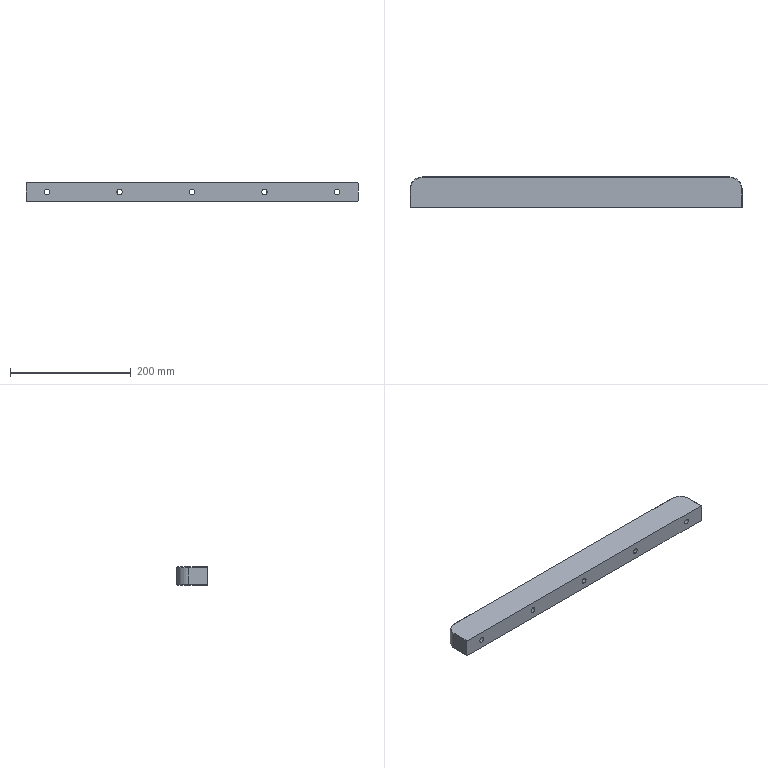Part | STEP file | TJ-DHQM-003-013 | 1 solid | 43 faces | box 550 x 50 x 30 mm | volume 789176 mm3 | cylinder 22 | plane 17 | cone 4 | commonest cylinder face diameters 9 x10 15 x10 40 x2
STEP:
#1=CARTESIAN_POINT('',(240.,25.,-7.5));
#2=VERTEX_POINT('',#1);
#3=CARTESIAN_POINT('',(240.,25.,7.5));
#4=VERTEX_POINT('',#3);
#5=CARTESIAN_POINT('',(240.,25.,0.));
#6=DIRECTION('',(0.,1.,0.));
#7=DIRECTION('',(0.,0.,1.));
#8=AXIS2_PLACEMENT_3D('',#5,#6,#7);
#9=CIRCLE('',#8,7.5);
#10=EDGE_CURVE('',#2,#4,#9,.T.);
#11=ORIENTED_EDGE('',*,*,#10,.F.);
#12=CARTESIAN_POINT('',(240.,50.,-7.5));
#13=VERTEX_POINT('',#12);
#14=CARTESIAN_POINT('',(240.,50.,-7.5));
#15=DIRECTION('',(0.,1.,0.));
#16=VECTOR('',#15,1000.);
#17=LINE('',#14,#16);
#18=EDGE_CURVE('',#2,#13,#17,.T.);
#19=ORIENTED_EDGE('',*,*,#18,.T.);
#20=CARTESIAN_POINT('',(240.,50.,7.5));
#21=VERTEX_POINT('',#20);
#22=CARTESIAN_POINT('',(240.,50.,0.));
#23=DIRECTION('',(0.,1.,0.));
#24=DIRECTION('',(0.,0.,1.));
#25=AXIS2_PLACEMENT_3D('',#22,#23,#24);
#26=CIRCLE('',#25,7.5);
#27=EDGE_CURVE('',#13,#21,#26,.T.);
#28=ORIENTED_EDGE('',*,*,#27,.T.);
#29=CARTESIAN_POINT('',(240.,50.,7.5));
#30=DIRECTION('',(0.,1.,0.));
#31=VECTOR('',#30,1000.);
#32=LINE('',#29,#31);
#33=EDGE_CURVE('',#4,#21,#32,.T.);
#34=ORIENTED_EDGE('',*,*,#33,.F.);
#35=EDGE_LOOP('',(#11,#19,#28,#34));
#36=FACE_OUTER_BOUND('',#35,.T.);
#37=CARTESIAN_POINT('',(240.,50.,0.));
#38=DIRECTION('',(0.,1.,0.));
#39=DIRECTION('',(0.,0.,1.));
#40=AXIS2_PLACEMENT_3D('',#37,#38,#39);
#41=CYLINDRICAL_SURFACE('',#40,7.5);
#42=ADVANCED_FACE('',(#36),#41,.F.);
#43=CARTESIAN_POINT('',(240.,0.,-4.5));
#44=VERTEX_POINT('',#43);
#45=CARTESIAN_POINT('',(240.,0.,4.5));
#46=VERTEX_POINT('',#45);
#47=CARTESIAN_POINT('',(240.,0.,0.));
#48=DIRECTION('',(0.,1.,0.));
#49=DIRECTION('',(0.,0.,1.));
#50=AXIS2_PLACEMENT_3D('',#47,#48,#49);
#51=CIRCLE('',#50,4.5);
#52=EDGE_CURVE('',#44,#46,#51,.T.);
#53=ORIENTED_EDGE('',*,*,#52,.F.);
#54=CARTESIAN_POINT('',(240.,25.,-4.5));
#55=VERTEX_POINT('',#54);
#56=CARTESIAN_POINT('',(240.,50.,-4.5));
#57=DIRECTION('',(0.,1.,0.));
#58=VECTOR('',#57,1000.);
#59=LINE('',#56,#58);
#60=EDGE_CURVE('',#44,#55,#59,.T.);
#61=ORIENTED_EDGE('',*,*,#60,.T.);
#62=CARTESIAN_POINT('',(240.,25.,4.5));
#63=VERTEX_POINT('',#62);
#64=CARTESIAN_POINT('',(240.,25.,0.));
#65=DIRECTION('',(0.,1.,0.));
#66=DIRECTION('',(0.,0.,1.));
#67=AXIS2_PLACEMENT_3D('',#64,#65,#66);
#68=CIRCLE('',#67,4.5);
#69=EDGE_CURVE('',#55,#63,#68,.T.);
#70=ORIENTED_EDGE('',*,*,#69,.T.);
#71=CARTESIAN_POINT('',(240.,50.,4.5));
#72=DIRECTION('',(0.,1.,0.));
#73=VECTOR('',#72,1000.);
#74=LINE('',#71,#73);
#75=EDGE_CURVE('',#46,#63,#74,.T.);
#76=ORIENTED_EDGE('',*,*,#75,.F.);
#77=EDGE_LOOP('',(#53,#61,#70,#76));
#78=FACE_OUTER_BOUND('',#77,.T.);
#79=CARTESIAN_POINT('',(240.,50.,0.));
#80=DIRECTION('',(0.,1.,0.));
#81=DIRECTION('',(0.,0.,1.));
#82=AXIS2_PLACEMENT_3D('',#79,#80,#81);
#83=CYLINDRICAL_SURFACE('',#82,4.5);
#84=ADVANCED_FACE('',(#78),#83,.F.);
#85=CARTESIAN_POINT('',(120.,25.,-7.5));
#86=VERTEX_POINT('',#85);
#87=CARTESIAN_POINT('',(120.,25.,7.5));
#88=VERTEX_POINT('',#87);
#89=CARTESIAN_POINT('',(120.,25.,0.));
#90=DIRECTION('',(0.,1.,0.));
#91=DIRECTION('',(0.,0.,1.));
#92=AXIS2_PLACEMENT_3D('',#89,#90,#91);
#93=CIRCLE('',#92,7.5);
#94=EDGE_CURVE('',#86,#88,#93,.T.);
#95=ORIENTED_EDGE('',*,*,#94,.F.);
#96=CARTESIAN_POINT('',(120.,50.,-7.5));
#97=VERTEX_POINT('',#96);
#98=CARTESIAN_POINT('',(120.,50.,-7.5));
#99=DIRECTION('',(0.,1.,0.));
#100=VECTOR('',#99,1000.);
#101=LINE('',#98,#100);
#102=EDGE_CURVE('',#86,#97,#101,.T.);
#103=ORIENTED_EDGE('',*,*,#102,.T.);
#104=CARTESIAN_POINT('',(120.,50.,7.5));
#105=VERTEX_POINT('',#104);
#106=CARTESIAN_POINT('',(120.,50.,0.));
#107=DIRECTION('',(0.,1.,0.));
#108=DIRECTION('',(0.,0.,1.));
#109=AXIS2_PLACEMENT_3D('',#106,#107,#108);
#110=CIRCLE('',#109,7.5);
#111=EDGE_CURVE('',#97,#105,#110,.T.);
#112=ORIENTED_EDGE('',*,*,#111,.T.);
#113=CARTESIAN_POINT('',(120.,50.,7.5));
#114=DIRECTION('',(0.,1.,0.));
#115=VECTOR('',#114,1000.);
#116=LINE('',#113,#115);
#117=EDGE_CURVE('',#88,#105,#116,.T.);
#118=ORIENTED_EDGE('',*,*,#117,.F.);
#119=EDGE_LOOP('',(#95,#103,#112,#118));
#120=FACE_OUTER_BOUND('',#119,.T.);
#121=CARTESIAN_POINT('',(120.,50.,0.));
#122=DIRECTION('',(0.,1.,0.));
#123=DIRECTION('',(0.,0.,1.));
#124=AXIS2_PLACEMENT_3D('',#121,#122,#123);
#125=CYLINDRICAL_SURFACE('',#124,7.5);
#126=ADVANCED_FACE('',(#120),#125,.F.);
#127=CARTESIAN_POINT('',(120.,0.,-4.5));
#128=VERTEX_POINT('',#127);
#129=CARTESIAN_POINT('',(120.,0.,4.5));
#130=VERTEX_POINT('',#129);
#131=CARTESIAN_POINT('',(120.,0.,0.));
#132=DIRECTION('',(0.,1.,0.));
#133=DIRECTION('',(0.,0.,1.));
#134=AXIS2_PLACEMENT_3D('',#131,#132,#133);
#135=CIRCLE('',#134,4.5);
#136=EDGE_CURVE('',#128,#130,#135,.T.);
#137=ORIENTED_EDGE('',*,*,#136,.F.);
#138=CARTESIAN_POINT('',(120.,25.,-4.5));
#139=VERTEX_POINT('',#138);
#140=CARTESIAN_POINT('',(120.,50.,-4.5));
#141=DIRECTION('',(0.,1.,0.));
#142=VECTOR('',#141,1000.);
#143=LINE('',#140,#142);
#144=EDGE_CURVE('',#128,#139,#143,.T.);
#145=ORIENTED_EDGE('',*,*,#144,.T.);
#146=CARTESIAN_POINT('',(120.,25.,4.5));
#147=VERTEX_POINT('',#146);
#148=CARTESIAN_POINT('',(120.,25.,0.));
#149=DIRECTION('',(0.,1.,0.));
#150=DIRECTION('',(0.,0.,1.));
#151=AXIS2_PLACEMENT_3D('',#148,#149,#150);
#152=CIRCLE('',#151,4.5);
#153=EDGE_CURVE('',#139,#147,#152,.T.);
#154=ORIENTED_EDGE('',*,*,#153,.T.);
#155=CARTESIAN_POINT('',(120.,50.,4.5));
#156=DIRECTION('',(0.,1.,0.));
#157=VECTOR('',#156,1000.);
#158=LINE('',#155,#157);
#159=EDGE_CURVE('',#130,#147,#158,.T.);
#160=ORIENTED_EDGE('',*,*,#159,.F.);
#161=EDGE_LOOP('',(#137,#145,#154,#160));
#162=FACE_OUTER_BOUND('',#161,.T.);
#163=CARTESIAN_POINT('',(120.,50.,0.));
#164=DIRECTION('',(0.,1.,0.));
#165=DIRECTION('',(0.,0.,1.));
#166=AXIS2_PLACEMENT_3D('',#163,#164,#165);
#167=CYLINDRICAL_SURFACE('',#166,4.5);
#168=ADVANCED_FACE('',(#162),#167,.F.);
#169=CARTESIAN_POINT('',(-240.,25.,-7.5));
#170=VERTEX_POINT('',#169);
#171=CARTESIAN_POINT('',(-240.,25.,7.5));
#172=VERTEX_POINT('',#171);
#173=CARTESIAN_POINT('',(-240.,25.,0.));
#174=DIRECTION('',(0.,1.,0.));
#175=DIRECTION('',(0.,0.,1.));
#176=AXIS2_PLACEMENT_3D('',#173,#174,#175);
#177=CIRCLE('',#176,7.5);
#178=EDGE_CURVE('',#170,#172,#177,.T.);
#179=ORIENTED_EDGE('',*,*,#178,.F.);
#180=CARTESIAN_POINT('',(-240.,50.,-7.5));
#181=VERTEX_POINT('',#180);
#182=CARTESIAN_POINT('',(-240.,50.,-7.5));
#183=DIRECTION('',(0.,1.,0.));
#184=VECTOR('',#183,1000.);
#185=LINE('',#182,#184);
#186=EDGE_CURVE('',#170,#181,#185,.T.);
#187=ORIENTED_EDGE('',*,*,#186,.T.);
#188=CARTESIAN_POINT('',(-240.,50.,7.5));
#189=VERTEX_POINT('',#188);
#190=CARTESIAN_POINT('',(-240.,50.,0.));
#191=DIRECTION('',(0.,1.,0.));
#192=DIRECTION('',(0.,0.,1.));
#193=AXIS2_PLACEMENT_3D('',#190,#191,#192);
#194=CIRCLE('',#193,7.5);
#195=EDGE_CURVE('',#181,#189,#194,.T.);
#196=ORIENTED_EDGE('',*,*,#195,.T.);
#197=CARTESIAN_POINT('',(-240.,50.,7.5));
#198=DIRECTION('',(0.,1.,0.));
#199=VECTOR('',#198,1000.);
#200=LINE('',#197,#199);
#201=EDGE_CURVE('',#172,#189,#200,.T.);
#202=ORIENTED_EDGE('',*,*,#201,.F.);
#203=EDGE_LOOP('',(#179,#187,#196,#202));
#204=FACE_OUTER_BOUND('',#203,.T.);
#205=CARTESIAN_POINT('',(-240.,50.,0.));
#206=DIRECTION('',(0.,1.,0.));
#207=DIRECTION('',(0.,0.,1.));
#208=AXIS2_PLACEMENT_3D('',#205,#206,#207);
#209=CYLINDRICAL_SURFACE('',#208,7.5);
#210=ADVANCED_FACE('',(#204),#209,.F.);
#211=CARTESIAN_POINT('',(-240.,0.,-4.5));
#212=VERTEX_POINT('',#211);
#213=CARTESIAN_POINT('',(-240.,0.,4.5));
#214=VERTEX_POINT('',#213);
#215=CARTESIAN_POINT('',(-240.,0.,0.));
#216=DIRECTION('',(0.,1.,0.));
#217=DIRECTION('',(0.,0.,1.));
#218=AXIS2_PLACEMENT_3D('',#215,#216,#217);
#219=CIRCLE('',#218,4.5);
#220=EDGE_CURVE('',#212,#214,#219,.T.);
#221=ORIENTED_EDGE('',*,*,#220,.F.);
#222=CARTESIAN_POINT('',(-240.,25.,-4.5));
#223=VERTEX_POINT('',#222);
#224=CARTESIAN_POINT('',(-240.,50.,-4.5));
#225=DIRECTION('',(0.,1.,0.));
#226=VECTOR('',#225,1000.);
#227=LINE('',#224,#226);
#228=EDGE_CURVE('',#212,#223,#227,.T.);
#229=ORIENTED_EDGE('',*,*,#228,.T.);
#230=CARTESIAN_POINT('',(-240.,25.,4.5));
#231=VERTEX_POINT('',#230);
#232=CARTESIAN_POINT('',(-240.,25.,0.));
#233=DIRECTION('',(0.,1.,0.));
#234=DIRECTION('',(0.,0.,1.));
#235=AXIS2_PLACEMENT_3D('',#232,#233,#234);
#236=CIRCLE('',#235,4.5);
#237=EDGE_CURVE('',#223,#231,#236,.T.);
#238=ORIENTED_EDGE('',*,*,#237,.T.);
#239=CARTESIAN_POINT('',(-240.,50.,4.5));
#240=DIRECTION('',(0.,1.,0.));
#241=VECTOR('',#240,1000.);
#242=LINE('',#239,#241);
#243=EDGE_CURVE('',#214,#231,#242,.T.);
#244=ORIENTED_EDGE('',*,*,#243,.F.);
#245=EDGE_LOOP('',(#221,#229,#238,#244));
#246=FACE_OUTER_BOUND('',#245,.T.);
#247=CARTESIAN_POINT('',(-240.,50.,0.));
#248=DIRECTION('',(0.,1.,0.));
#249=DIRECTION('',(0.,0.,1.));
#250=AXIS2_PLACEMENT_3D('',#247,#248,#249);
#251=CYLINDRICAL_SURFACE('',#250,4.5);
#252=ADVANCED_FACE('',(#246),#251,.F.);
#253=CARTESIAN_POINT('',(-120.,25.,-7.5));
#254=VERTEX_POINT('',#253);
#255=CARTESIAN_POINT('',(-120.,25.,7.5));
#256=VERTEX_POINT('',#255);
#257=CARTESIAN_POINT('',(-120.,25.,0.));
#258=DIRECTION('',(0.,1.,0.));
#259=DIRECTION('',(0.,0.,1.));
#260=AXIS2_PLACEMENT_3D('',#257,#258,#259);
#261=CIRCLE('',#260,7.5);
#262=EDGE_CURVE('',#254,#256,#261,.T.);
#263=ORIENTED_EDGE('',*,*,#262,.F.);
#264=CARTESIAN_POINT('',(-120.,50.,-7.5));
#265=VERTEX_POINT('',#264);
#266=CARTESIAN_POINT('',(-120.,50.,-7.5));
#267=DIRECTION('',(0.,1.,0.));
#268=VECTOR('',#267,1000.);
#269=LINE('',#266,#268);
#270=EDGE_CURVE('',#254,#265,#269,.T.);
#271=ORIENTED_EDGE('',*,*,#270,.T.);
#272=CARTESIAN_POINT('',(-120.,50.,7.5));
#273=VERTEX_POINT('',#272);
#274=CARTESIAN_POINT('',(-120.,50.,0.));
#275=DIRECTION('',(0.,1.,0.));
#276=DIRECTION('',(0.,0.,1.));
#277=AXIS2_PLACEMENT_3D('',#274,#275,#276);
#278=CIRCLE('',#277,7.5);
#279=EDGE_CURVE('',#265,#273,#278,.T.);
#280=ORIENTED_EDGE('',*,*,#279,.T.);
#281=CARTESIAN_POINT('',(-120.,50.,7.5));
#282=DIRECTION('',(0.,1.,0.));
#283=VECTOR('',#282,1000.);
#284=LINE('',#281,#283);
#285=EDGE_CURVE('',#256,#273,#284,.T.);
#286=ORIENTED_EDGE('',*,*,#285,.F.);
#287=EDGE_LOOP('',(#263,#271,#280,#286));
#288=FACE_OUTER_BOUND('',#287,.T.);
#289=CARTESIAN_POINT('',(-120.,50.,0.));
#290=DIRECTION('',(0.,1.,0.));
#291=DIRECTION('',(0.,0.,1.));
#292=AXIS2_PLACEMENT_3D('',#289,#290,#291);
#293=CYLINDRICAL_SURFACE('',#292,7.5);
#294=ADVANCED_FACE('',(#288),#293,.F.);
#295=CARTESIAN_POINT('',(-120.,0.,-4.5));
#296=VERTEX_POINT('',#295);
#297=CARTESIAN_POINT('',(-120.,0.,4.5));
#298=VERTEX_POINT('',#297);
#299=CARTESIAN_POINT('',(-120.,0.,0.));
#300=DIRECTION('',(0.,1.,0.));
#301=DIRECTION('',(0.,0.,1.));
#302=AXIS2_PLACEMENT_3D('',#299,#300,#301);
#303=CIRCLE('',#302,4.5);
#304=EDGE_CURVE('',#296,#298,#303,.T.);
#305=ORIENTED_EDGE('',*,*,#304,.F.);
#306=CARTESIAN_POINT('',(-120.,25.,-4.5));
#307=VERTEX_POINT('',#306);
#308=CARTESIAN_POINT('',(-120.,50.,-4.5));
#309=DIRECTION('',(0.,1.,0.));
#310=VECTOR('',#309,1000.);
#311=LINE('',#308,#310);
#312=EDGE_CURVE('',#296,#307,#311,.T.);
#313=ORIENTED_EDGE('',*,*,#312,.T.);
#314=CARTESIAN_POINT('',(-120.,25.,4.5));
#315=VERTEX_POINT('',#314);
#316=CARTESIAN_POINT('',(-120.,25.,0.));
#317=DIRECTION('',(0.,1.,0.));
#318=DIRECTION('',(0.,0.,1.));
#319=AXIS2_PLACEMENT_3D('',#316,#317,#318);
#320=CIRCLE('',#319,4.5);
#321=EDGE_CURVE('',#307,#315,#320,.T.);
#322=ORIENTED_EDGE('',*,*,#321,.T.);
#323=CARTESIAN_POINT('',(-120.,50.,4.5));
#324=DIRECTION('',(0.,1.,0.));
#325=VECTOR('',#324,1000.);
#326=LINE('',#323,#325);
#327=EDGE_CURVE('',#298,#315,#326,.T.);
#328=ORIENTED_EDGE('',*,*,#327,.F.);
#329=EDGE_LOOP('',(#305,#313,#322,#328));
#330=FACE_OUTER_BOUND('',#329,.T.);
#331=CARTESIAN_POINT('',(-120.,50.,0.));
#332=DIRECTION('',(0.,1.,0.));
#333=DIRECTION('',(0.,0.,1.));
#334=AXIS2_PLACEMENT_3D('',#331,#332,#333);
#335=CYLINDRICAL_SURFACE('',#334,4.5);
#336=ADVANCED_FACE('',(#330),#335,.F.);
#337=CARTESIAN_POINT('',(0.,25.,-7.5));
#338=VERTEX_POINT('',#337);
#339=CARTESIAN_POINT('',(0.,25.,7.5));
#340=VERTEX_POINT('',#339);
#341=CARTESIAN_POINT('',(0.,25.,0.));
#342=DIRECTION('',(0.,1.,0.));
#343=DIRECTION('',(0.,0.,1.));
#344=AXIS2_PLACEMENT_3D('',#341,#342,#343);
#345=CIRCLE('',#344,7.5);
#346=EDGE_CURVE('',#338,#340,#345,.T.);
#347=ORIENTED_EDGE('',*,*,#346,.F.);
#348=CARTESIAN_POINT('',(0.,50.,-7.5));
#349=VERTEX_POINT('',#348);
#350=CARTESIAN_POINT('',(0.,50.,-7.5));
#351=DIRECTION('',(0.,1.,0.));
#352=VECTOR('',#351,1000.);
#353=LINE('',#350,#352);
#354=EDGE_CURVE('',#338,#349,#353,.T.);
#355=ORIENTED_EDGE('',*,*,#354,.T.);
#356=CARTESIAN_POINT('',(0.,50.,7.5));
#357=VERTEX_POINT('',#356);
#358=CARTESIAN_POINT('',(0.,50.,0.));
#359=DIRECTION('',(0.,1.,0.));
#360=DIRECTION('',(0.,0.,1.));
#361=AXIS2_PLACEMENT_3D('',#358,#359,#360);
#362=CIRCLE('',#361,7.5);
#363=EDGE_CURVE('',#349,#357,#362,.T.);
#364=ORIENTED_EDGE('',*,*,#363,.T.);
#365=CARTESIAN_POINT('',(0.,50.,7.5));
#366=DIRECTION('',(0.,1.,0.));
#367=VECTOR('',#366,1000.);
#368=LINE('',#365,#367);
#369=EDGE_CURVE('',#340,#357,#368,.T.);
#370=ORIENTED_EDGE('',*,*,#369,.F.);
#371=EDGE_LOOP('',(#347,#355,#364,#370));
#372=FACE_OUTER_BOUND('',#371,.T.);
#373=CARTESIAN_POINT('',(0.,50.,0.));
#374=DIRECTION('',(0.,1.,0.));
#375=DIRECTION('',(0.,0.,1.));
#376=AXIS2_PLACEMENT_3D('',#373,#374,#375);
#377=CYLINDRICAL_SURFACE('',#376,7.5);
#378=ADVANCED_FACE('',(#372),#377,.F.);
#379=CARTESIAN_POINT('',(0.,0.,-4.5));
#380=VERTEX_POINT('',#379);
#381=CARTESIAN_POINT('',(0.,0.,4.5));
#382=VERTEX_POINT('',#381);
#383=CARTESIAN_POINT('',(0.,0.,0.));
#384=DIRECTION('',(0.,1.,0.));
#385=DIRECTION('',(0.,0.,1.));
#386=AXIS2_PLACEMENT_3D('',#383,#384,#385);
#387=CIRCLE('',#386,4.5);
#388=EDGE_CURVE('',#380,#382,#387,.T.);
#389=ORIENTED_EDGE('',*,*,#388,.F.);
#390=CARTESIAN_POINT('',(0.,25.,-4.5));
#391=VERTEX_POINT('',#390);
#392=CARTESIAN_POINT('',(0.,50.,-4.5));
#393=DIRECTION('',(0.,1.,0.));
#394=VECTOR('',#393,1000.);
#395=LINE('',#392,#394);
#396=EDGE_CURVE('',#380,#391,#395,.T.);
#397=ORIENTED_EDGE('',*,*,#396,.T.);
#398=CARTESIAN_POINT('',(0.,25.,4.5));
#399=VERTEX_POINT('',#398);
#400=CARTESIAN_POINT('',(0.,25.,0.));
#401=DIRECTION('',(0.,1.,0.));
#402=DIRECTION('',(0.,0.,1.));
#403=AXIS2_PLACEMENT_3D('',#400,#401,#402);
#404=CIRCLE('',#403,4.5);
#405=EDGE_CURVE('',#391,#399,#404,.T.);
#406=ORIENTED_EDGE('',*,*,#405,.T.);
#407=CARTESIAN_POINT('',(0.,50.,4.5));
#408=DIRECTION('',(0.,1.,0.));
#409=VECTOR('',#408,1000.);
#410=LINE('',#407,#409);
#411=EDGE_CURVE('',#382,#399,#410,.T.);
#412=ORIENTED_EDGE('',*,*,#411,.F.);
#413=EDGE_LOOP('',(#389,#397,#406,#412));
#414=FACE_OUTER_BOUND('',#413,.T.);
#415=CARTESIAN_POINT('',(0.,50.,0.));
#416=DIRECTION('',(0.,1.,0.));
#417=DIRECTION('',(0.,0.,1.));
#418=AXIS2_PLACEMENT_3D('',#415,#416,#417);
#419=CYLINDRICAL_SURFACE('',#418,4.5);
#420=ADVANCED_FACE('',(#414),#419,.F.);
#421=CARTESIAN_POINT('',(-275.,30.,14.));
#422=VERTEX_POINT('',#421);
#423=CARTESIAN_POINT('',(-275.,30.,-14.));
#424=VERTEX_POINT('',#423);
#425=CARTESIAN_POINT('',(-275.,30.,-15.));
#426=DIRECTION('',(0.,0.,-1.));
#427=VECTOR('',#426,1000.);
#428=LINE('',#425,#427);
#429=EDGE_CURVE('',#422,#424,#428,.T.);
#430=ORIENTED_EDGE('',*,*,#429,.T.);
#431=CARTESIAN_POINT('',(-275.,0.,-14.));
#432=VERTEX_POINT('',#431);
#433=CARTESIAN_POINT('',(-275.,0.,-14.));
#434=DIRECTION('',(0.,-1.,0.));
#435=VECTOR('',#434,1000.);
#436=LINE('',#433,#435);
#437=EDGE_CURVE('',#424,#432,#436,.T.);
#438=ORIENTED_EDGE('',*,*,#437,.T.);
#439=CARTESIAN_POINT('',(-275.,0.,14.));
#440=VERTEX_POINT('',#439);
#441=CARTESIAN_POINT('',(-275.,0.,-15.));
#442=DIRECTION('',(0.,0.,1.));
#443=VECTOR('',#442,1000.);
#444=LINE('',#441,#443);
#445=EDGE_CURVE('',#432,#440,#444,.T.);
#446=ORIENTED_EDGE('',*,*,#445,.T.);
#447=CARTESIAN_POINT('',(-275.,30.,14.));
#448=DIRECTION('',(0.,1.,0.));
#449=VECTOR('',#448,1000.);
#450=LINE('',#447,#449);
#451=EDGE_CURVE('',#440,#422,#450,.T.);
#452=ORIENTED_EDGE('',*,*,#451,.T.);
#453=EDGE_LOOP('',(#430,#438,#446,#452));
#454=FACE_OUTER_BOUND('',#453,.T.);
#455=CARTESIAN_POINT('',(-275.,0.,-15.));
#456=DIRECTION('',(-1.,0.,0.));
#457=DIRECTION('',(0.,0.,1.));
#458=AXIS2_PLACEMENT_3D('',#455,#456,#457);
#459=PLANE('',#458);
#460=ADVANCED_FACE('',(#454),#459,.T.);
#461=CARTESIAN_POINT('',(240.,50.,0.));
#462=DIRECTION('',(0.,1.,0.));
#463=DIRECTION('',(0.,0.,1.));
#464=AXIS2_PLACEMENT_3D('',#461,#462,#463);
#465=CIRCLE('',#464,7.5);
#466=EDGE_CURVE('',#21,#13,#465,.T.);
#467=ORIENTED_EDGE('',*,*,#466,.F.);
#468=ORIENTED_EDGE('',*,*,#27,.F.);
#469=EDGE_LOOP('',(#467,#468));
#470=FACE_BOUND('',#469,.T.);
#471=CARTESIAN_POINT('',(120.,50.,0.));
#472=DIRECTION('',(0.,1.,0.));
#473=DIRECTION('',(0.,0.,1.));
#474=AXIS2_PLACEMENT_3D('',#471,#472,#473);
#475=CIRCLE('',#474,7.5);
#476=EDGE_CURVE('',#105,#97,#475,.T.);
#477=ORIENTED_EDGE('',*,*,#476,.F.);
#478=ORIENTED_EDGE('',*,*,#111,.F.);
#479=EDGE_LOOP('',(#477,#478));
#480=FACE_BOUND('',#479,.T.);
#481=CARTESIAN_POINT('',(-240.,50.,0.));
#482=DIRECTION('',(0.,1.,0.));
#483=DIRECTION('',(0.,0.,1.));
#484=AXIS2_PLACEMENT_3D('',#481,#482,#483);
#485=CIRCLE('',#484,7.5);
#486=EDGE_CURVE('',#189,#181,#485,.T.);
#487=ORIENTED_EDGE('',*,*,#486,.F.);
#488=ORIENTED_EDGE('',*,*,#195,.F.);
#489=EDGE_LOOP('',(#487,#488));
#490=FACE_BOUND('',#489,.T.);
#491=CARTESIAN_POINT('',(-120.,50.,0.));
#492=DIRECTION('',(0.,1.,0.));
#493=DIRECTION('',(0.,0.,1.));
#494=AXIS2_PLACEMENT_3D('',#491,#492,#493);
#495=CIRCLE('',#494,7.5);
#496=EDGE_CURVE('',#273,#265,#495,.T.);
#497=ORIENTED_EDGE('',*,*,#496,.F.);
#498=ORIENTED_EDGE('',*,*,#279,.F.);
#499=EDGE_LOOP('',(#497,#498));
#500=FACE_BOUND('',#499,.T.);
#501=CARTESIAN_POINT('',(0.,50.,0.));
#502=DIRECTION('',(0.,1.,0.));
#503=DIRECTION('',(0.,0.,1.));
#504=AXIS2_PLACEMENT_3D('',#501,#502,#503);
#505=CIRCLE('',#504,7.5);
#506=EDGE_CURVE('',#357,#349,#505,.T.);
#507=ORIENTED_EDGE('',*,*,#506,.F.);
#508=ORIENTED_EDGE('',*,*,#363,.F.);
#509=EDGE_LOOP('',(#507,#508));
#510=FACE_BOUND('',#509,.T.);
#511=CARTESIAN_POINT('',(255.,50.,14.));
#512=VERTEX_POINT('',#511);
#513=CARTESIAN_POINT('',(255.,50.,-14.));
#514=VERTEX_POINT('',#513);
#515=CARTESIAN_POINT('',(255.,50.,-15.));
#516=DIRECTION('',(0.,0.,-1.));
#517=VECTOR('',#516,1000.);
#518=LINE('',#515,#517);
#519=EDGE_CURVE('',#512,#514,#518,.T.);
#520=ORIENTED_EDGE('',*,*,#519,.T.);
#521=CARTESIAN_POINT('',(-255.,50.,-14.));
#522=VERTEX_POINT('',#521);
#523=CARTESIAN_POINT('',(-275.,50.,-14.));
#524=DIRECTION('',(-1.,0.,0.));
#525=VECTOR('',#524,1000.);
#526=LINE('',#523,#525);
#527=EDGE_CURVE('',#514,#522,#526,.T.);
#528=ORIENTED_EDGE('',*,*,#527,.T.);
#529=CARTESIAN_POINT('',(-255.,50.,14.));
#530=VERTEX_POINT('',#529);
#531=CARTESIAN_POINT('',(-255.,50.,-15.));
#532=DIRECTION('',(0.,0.,1.));
#533=VECTOR('',#532,1000.);
#534=LINE('',#531,#533);
#535=EDGE_CURVE('',#522,#530,#534,.T.);
#536=ORIENTED_EDGE('',*,*,#535,.T.);
#537=CARTESIAN_POINT('',(255.,50.,14.));
#538=DIRECTION('',(1.,0.,0.));
#539=VECTOR('',#538,1000.);
#540=LINE('',#537,#539);
#541=EDGE_CURVE('',#530,#512,#540,.T.);
#542=ORIENTED_EDGE('',*,*,#541,.T.);
#543=EDGE_LOOP('',(#520,#528,#536,#542));
#544=FACE_OUTER_BOUND('',#543,.T.);
#545=CARTESIAN_POINT('',(-275.,50.,-15.));
#546=DIRECTION('',(0.,1.,0.));
#547=DIRECTION('',(0.,0.,1.));
#548=AXIS2_PLACEMENT_3D('',#545,#546,#547);
#549=PLANE('',#548);
#550=ADVANCED_FACE('',(#470,#480,#490,#500,#510,#544),#549,.T.);
#551=CARTESIAN_POINT('',(275.,0.,-14.));
#552=VERTEX_POINT('',#551);
#553=CARTESIAN_POINT('',(275.,0.,14.));
#554=VERTEX_POINT('',#553);
#555=CARTESIAN_POINT('',(275.,0.,-15.));
#556=DIRECTION('',(0.,0.,1.));
#557=VECTOR('',#556,1000.);
#558=LINE('',#555,#557);
#559=EDGE_CURVE('',#552,#554,#558,.T.);
#560=ORIENTED_EDGE('',*,*,#559,.F.);
#561=CARTESIAN_POINT('',(275.,30.,-14.));
#562=VERTEX_POINT('',#561);
#563=CARTESIAN_POINT('',(275.,0.,-14.));
#564=DIRECTION('',(0.,1.,0.));
#565=VECTOR('',#564,1000.);
#566=LINE('',#563,#565);
#567=EDGE_CURVE('',#552,#562,#566,.T.);
#568=ORIENTED_EDGE('',*,*,#567,.T.);
#569=CARTESIAN_POINT('',(275.,30.,14.));
#570=VERTEX_POINT('',#569);
#571=CARTESIAN_POINT('',(275.,30.,-15.));
#572=DIRECTION('',(0.,0.,1.));
#573=VECTOR('',#572,1000.);
#574=LINE('',#571,#573);
#575=EDGE_CURVE('',#562,#570,#574,.T.);
#576=ORIENTED_EDGE('',*,*,#575,.T.);
#577=CARTESIAN_POINT('',(275.,0.,14.));
#578=DIRECTION('',(0.,-1.,0.));
#579=VECTOR('',#578,1000.);
#580=LINE('',#577,#579);
#581=EDGE_CURVE('',#570,#554,#580,.T.);
#582=ORIENTED_EDGE('',*,*,#581,.T.);
#583=EDGE_LOOP('',(#560,#568,#576,#582));
#584=FACE_OUTER_BOUND('',#583,.T.);
#585=CARTESIAN_POINT('',(275.,0.,-15.));
#586=DIRECTION('',(1.,0.,0.));
#587=DIRECTION('',(0.,0.,-1.));
#588=AXIS2_PLACEMENT_3D('',#585,#586,#587);
#589=PLANE('',#588);
#590=ADVANCED_FACE('',(#584),#589,.T.);
#591=CARTESIAN_POINT('',(240.,0.,0.));
#592=DIRECTION('',(0.,1.,0.));
#593=DIRECTION('',(0.,0.,1.));
#594=AXIS2_PLACEMENT_3D('',#591,#592,#593);
#595=CIRCLE('',#594,4.5);
#596=EDGE_CURVE('',#46,#44,#595,.T.);
#597=ORIENTED_EDGE('',*,*,#596,.T.);
#598=ORIENTED_EDGE('',*,*,#52,.T.);
#599=EDGE_LOOP('',(#597,#598));
#600=FACE_BOUND('',#599,.T.);
#601=CARTESIAN_POINT('',(120.,0.,0.));
#602=DIRECTION('',(0.,1.,0.));
#603=DIRECTION('',(0.,0.,1.));
#604=AXIS2_PLACEMENT_3D('',#601,#602,#603);
#605=CIRCLE('',#604,4.5);
#606=EDGE_CURVE('',#130,#128,#605,.T.);
#607=ORIENTED_EDGE('',*,*,#606,.T.);
#608=ORIENTED_EDGE('',*,*,#136,.T.);
#609=EDGE_LOOP('',(#607,#608));
#610=FACE_BOUND('',#609,.T.);
#611=CARTESIAN_POINT('',(-240.,0.,0.));
#612=DIRECTION('',(0.,1.,0.));
#613=DIRECTION('',(0.,0.,1.));
#614=AXIS2_PLACEMENT_3D('',#611,#612,#613);
#615=CIRCLE('',#614,4.5);
#616=EDGE_CURVE('',#214,#212,#615,.T.);
#617=ORIENTED_EDGE('',*,*,#616,.T.);
#618=ORIENTED_EDGE('',*,*,#220,.T.);
#619=EDGE_LOOP('',(#617,#618));
#620=FACE_BOUND('',#619,.T.);
#621=CARTESIAN_POINT('',(-120.,0.,0.));
#622=DIRECTION('',(0.,1.,0.));
#623=DIRECTION('',(0.,0.,1.));
#624=AXIS2_PLACEMENT_3D('',#621,#622,#623);
#625=CIRCLE('',#624,4.5);
#626=EDGE_CURVE('',#298,#296,#625,.T.);
#627=ORIENTED_EDGE('',*,*,#626,.T.);
#628=ORIENTED_EDGE('',*,*,#304,.T.);
#629=EDGE_LOOP('',(#627,#628));
#630=FACE_BOUND('',#629,.T.);
#631=CARTESIAN_POINT('',(0.,0.,0.));
#632=DIRECTION('',(0.,1.,0.));
#633=DIRECTION('',(0.,0.,1.));
#634=AXIS2_PLACEMENT_3D('',#631,#632,#633);
#635=CIRCLE('',#634,4.5);
#636=EDGE_CURVE('',#382,#380,#635,.T.);
#637=ORIENTED_EDGE('',*,*,#636,.T.);
#638=ORIENTED_EDGE('',*,*,#388,.T.);
#639=EDGE_LOOP('',(#637,#638));
#640=FACE_BOUND('',#639,.T.);
#641=CARTESIAN_POINT('',(-274.,0.,-15.));
#642=VERTEX_POINT('',#641);
#643=CARTESIAN_POINT('',(274.,0.,-15.));
#644=VERTEX_POINT('',#643);
#645=CARTESIAN_POINT('',(275.,0.,-15.));
#646=DIRECTION('',(1.,0.,0.));
#647=VECTOR('',#646,1000.);
#648=LINE('',#645,#647);
#649=EDGE_CURVE('',#642,#644,#648,.T.);
#650=ORIENTED_EDGE('',*,*,#649,.T.);
#651=CARTESIAN_POINT('',(274.5,0.,-14.5));
#652=DIRECTION('',(0.7071,0.,0.7071));
#653=VECTOR('',#652,1000.);
#654=LINE('',#651,#653);
#655=EDGE_CURVE('',#644,#552,#654,.T.);
#656=ORIENTED_EDGE('',*,*,#655,.T.);
#657=ORIENTED_EDGE('',*,*,#559,.T.);
#658=CARTESIAN_POINT('',(274.,0.,15.));
#659=VERTEX_POINT('',#658);
#660=CARTESIAN_POINT('',(289.5,0.,-0.5));
#661=DIRECTION('',(-0.7071,0.,0.7071));
#662=VECTOR('',#661,1000.);
#663=LINE('',#660,#662);
#664=EDGE_CURVE('',#554,#659,#663,.T.);
#665=ORIENTED_EDGE('',*,*,#664,.T.);
#666=CARTESIAN_POINT('',(-274.,0.,15.));
#667=VERTEX_POINT('',#666);
#668=CARTESIAN_POINT('',(275.,0.,15.));
#669=DIRECTION('',(1.,0.,0.));
#670=VECTOR('',#669,1000.);
#671=LINE('',#668,#670);
#672=EDGE_CURVE('',#667,#659,#671,.T.);
#673=ORIENTED_EDGE('',*,*,#672,.F.);
#674=CARTESIAN_POINT('',(-14.5,0.,274.5));
#675=DIRECTION('',(-0.7071,0.,-0.7071));
#676=VECTOR('',#675,1000.);
#677=LINE('',#674,#676);
#678=EDGE_CURVE('',#667,#440,#677,.T.);
#679=ORIENTED_EDGE('',*,*,#678,.T.);
#680=ORIENTED_EDGE('',*,*,#445,.F.);
#681=CARTESIAN_POINT('',(0.5,0.,-289.5));
#682=DIRECTION('',(0.7071,0.,-0.7071));
#683=VECTOR('',#682,1000.);
#684=LINE('',#681,#683);
#685=EDGE_CURVE('',#432,#642,#684,.T.);
#686=ORIENTED_EDGE('',*,*,#685,.T.);
#687=EDGE_LOOP('',(#650,#656,#657,#665,#673,#679,#680,#686));
#688=FACE_OUTER_BOUND('',#687,.T.);
#689=CARTESIAN_POINT('',(275.,0.,-15.));
#690=DIRECTION('',(0.,-1.,0.));
#691=DIRECTION('',(0.,0.,-1.));
#692=AXIS2_PLACEMENT_3D('',#689,#690,#691);
#693=PLANE('',#692);
#694=ADVANCED_FACE('',(#600,#610,#620,#630,#640,#688),#693,.T.);
#695=CARTESIAN_POINT('',(255.,49.,-15.));
#696=VERTEX_POINT('',#695);
#697=CARTESIAN_POINT('',(274.,30.,-15.));
#698=VERTEX_POINT('',#697);
#699=CARTESIAN_POINT('',(255.,30.,-15.));
#700=DIRECTION('',(0.,0.,-1.));
#701=DIRECTION('',(-1.,0.,0.));
#702=AXIS2_PLACEMENT_3D('',#699,#700,#701);
#703=CIRCLE('',#702,19.);
#704=EDGE_CURVE('',#696,#698,#703,.T.);
#705=ORIENTED_EDGE('',*,*,#704,.T.);
#706=CARTESIAN_POINT('',(274.,0.,-15.));
#707=DIRECTION('',(0.,-1.,0.));
#708=VECTOR('',#707,1000.);
#709=LINE('',#706,#708);
#710=EDGE_CURVE('',#698,#644,#709,.T.);
#711=ORIENTED_EDGE('',*,*,#710,.T.);
#712=ORIENTED_EDGE('',*,*,#649,.F.);
#713=CARTESIAN_POINT('',(-274.,30.,-15.));
#714=VERTEX_POINT('',#713);
#715=CARTESIAN_POINT('',(-274.,0.,-15.));
#716=DIRECTION('',(0.,1.,0.));
#717=VECTOR('',#716,1000.);
#718=LINE('',#715,#717);
#719=EDGE_CURVE('',#642,#714,#718,.T.);
#720=ORIENTED_EDGE('',*,*,#719,.T.);
#721=CARTESIAN_POINT('',(-255.,49.,-15.));
#722=VERTEX_POINT('',#721);
#723=CARTESIAN_POINT('',(-255.,30.,-15.));
#724=DIRECTION('',(0.,0.,-1.));
#725=DIRECTION('',(-1.,0.,0.));
#726=AXIS2_PLACEMENT_3D('',#723,#724,#725);
#727=CIRCLE('',#726,19.);
#728=EDGE_CURVE('',#714,#722,#727,.T.);
#729=ORIENTED_EDGE('',*,*,#728,.T.);
#730=CARTESIAN_POINT('',(0.,49.,-15.));
#731=DIRECTION('',(1.,0.,0.));
#732=VECTOR('',#731,1000.);
#733=LINE('',#730,#732);
#734=EDGE_CURVE('',#722,#696,#733,.T.);
#735=ORIENTED_EDGE('',*,*,#734,.T.);
#736=EDGE_LOOP('',(#705,#711,#712,#720,#729,#735));
#737=FACE_OUTER_BOUND('',#736,.T.);
#738=CARTESIAN_POINT('',(0.,0.,-15.));
#739=DIRECTION('',(0.,0.,-1.));
#740=DIRECTION('',(-1.,0.,0.));
#741=AXIS2_PLACEMENT_3D('',#738,#739,#740);
#742=PLANE('',#741);
#743=ADVANCED_FACE('',(#737),#742,.T.);
#744=ORIENTED_EDGE('',*,*,#672,.T.);
#745=CARTESIAN_POINT('',(274.,30.,15.));
#746=VERTEX_POINT('',#745);
#747=CARTESIAN_POINT('',(274.,30.,15.));
#748=DIRECTION('',(0.,1.,0.));
#749=VECTOR('',#748,1000.);
#750=LINE('',#747,#749);
#751=EDGE_CURVE('',#659,#746,#750,.T.);
#752=ORIENTED_EDGE('',*,*,#751,.T.);
#753=CARTESIAN_POINT('',(255.,49.,15.));
#754=VERTEX_POINT('',#753);
#755=CARTESIAN_POINT('',(255.,30.,15.));
#756=DIRECTION('',(0.,0.,1.));
#757=DIRECTION('',(-1.,0.,0.));
#758=AXIS2_PLACEMENT_3D('',#755,#756,#757);
#759=CIRCLE('',#758,19.);
#760=EDGE_CURVE('',#746,#754,#759,.T.);
#761=ORIENTED_EDGE('',*,*,#760,.T.);
#762=CARTESIAN_POINT('',(-255.,49.,15.));
#763=VERTEX_POINT('',#762);
#764=CARTESIAN_POINT('',(-255.,49.,15.));
#765=DIRECTION('',(-1.,0.,0.));
#766=VECTOR('',#765,1000.);
#767=LINE('',#764,#766);
#768=EDGE_CURVE('',#754,#763,#767,.T.);
#769=ORIENTED_EDGE('',*,*,#768,.T.);
#770=CARTESIAN_POINT('',(-274.,30.,15.));
#771=VERTEX_POINT('',#770);
#772=CARTESIAN_POINT('',(-255.,30.,15.));
#773=DIRECTION('',(0.,0.,1.));
#774=DIRECTION('',(-1.,0.,0.));
#775=AXIS2_PLACEMENT_3D('',#772,#773,#774);
#776=CIRCLE('',#775,19.);
#777=EDGE_CURVE('',#763,#771,#776,.T.);
#778=ORIENTED_EDGE('',*,*,#777,.T.);
#779=CARTESIAN_POINT('',(-274.,0.,15.));
#780=DIRECTION('',(0.,-1.,0.));
#781=VECTOR('',#780,1000.);
#782=LINE('',#779,#781);
#783=EDGE_CURVE('',#771,#667,#782,.T.);
#784=ORIENTED_EDGE('',*,*,#783,.T.);
#785=EDGE_LOOP('',(#744,#752,#761,#769,#778,#784));
#786=FACE_OUTER_BOUND('',#785,.T.);
#787=CARTESIAN_POINT('',(0.,0.,15.));
#788=DIRECTION('',(0.,0.,-1.));
#789=DIRECTION('',(-1.,0.,0.));
#790=AXIS2_PLACEMENT_3D('',#787,#788,#789);
#791=PLANE('',#790);
#792=ADVANCED_FACE('',(#786),#791,.F.);
#793=ORIENTED_EDGE('',*,*,#396,.F.);
#794=ORIENTED_EDGE('',*,*,#636,.F.);
#795=ORIENTED_EDGE('',*,*,#411,.T.);
#796=CARTESIAN_POINT('',(0.,25.,0.));
#797=DIRECTION('',(0.,1.,0.));
#798=DIRECTION('',(0.,0.,1.));
#799=AXIS2_PLACEMENT_3D('',#796,#797,#798);
#800=CIRCLE('',#799,4.5);
#801=EDGE_CURVE('',#399,#391,#800,.T.);
#802=ORIENTED_EDGE('',*,*,#801,.T.);
#803=EDGE_LOOP('',(#793,#794,#795,#802));
#804=FACE_OUTER_BOUND('',#803,.T.);
#805=CARTESIAN_POINT('',(0.,50.,0.));
#806=DIRECTION('',(0.,1.,0.));
#807=DIRECTION('',(0.,0.,1.));
#808=AXIS2_PLACEMENT_3D('',#805,#806,#807);
#809=CYLINDRICAL_SURFACE('',#808,4.5);
#810=ADVANCED_FACE('',(#804),#809,.F.);
#811=ORIENTED_EDGE('',*,*,#801,.F.);
#812=ORIENTED_EDGE('',*,*,#405,.F.);
#813=EDGE_LOOP('',(#811,#812));
#814=FACE_BOUND('',#813,.T.);
#815=CARTESIAN_POINT('',(0.,25.,0.));
#816=DIRECTION('',(0.,1.,0.));
#817=DIRECTION('',(0.,0.,1.));
#818=AXIS2_PLACEMENT_3D('',#815,#816,#817);
#819=CIRCLE('',#818,7.5);
#820=EDGE_CURVE('',#340,#338,#819,.T.);
#821=ORIENTED_EDGE('',*,*,#820,.T.);
#822=ORIENTED_EDGE('',*,*,#346,.T.);
#823=EDGE_LOOP('',(#821,#822));
#824=FACE_OUTER_BOUND('',#823,.T.);
#825=CARTESIAN_POINT('',(4.5,25.,0.));
#826=DIRECTION('',(0.,-1.,0.));
#827=DIRECTION('',(0.,0.,-1.));
#828=AXIS2_PLACEMENT_3D('',#825,#826,#827);
#829=PLANE('',#828);
#830=ADVANCED_FACE('',(#814,#824),#829,.F.);
#831=ORIENTED_EDGE('',*,*,#354,.F.);
#832=ORIENTED_EDGE('',*,*,#820,.F.);
#833=ORIENTED_EDGE('',*,*,#369,.T.);
#834=ORIENTED_EDGE('',*,*,#506,.T.);
#835=EDGE_LOOP('',(#831,#832,#833,#834));
#836=FACE_OUTER_BOUND('',#835,.T.);
#837=CARTESIAN_POINT('',(0.,50.,0.));
#838=DIRECTION('',(0.,1.,0.));
#839=DIRECTION('',(0.,0.,1.));
#840=AXIS2_PLACEMENT_3D('',#837,#838,#839);
#841=CYLINDRICAL_SURFACE('',#840,7.5);
#842=ADVANCED_FACE('',(#836),#841,.F.);
#843=ORIENTED_EDGE('',*,*,#312,.F.);
#844=ORIENTED_EDGE('',*,*,#626,.F.);
#845=ORIENTED_EDGE('',*,*,#327,.T.);
#846=CARTESIAN_POINT('',(-120.,25.,0.));
#847=DIRECTION('',(0.,1.,0.));
#848=DIRECTION('',(0.,0.,1.));
#849=AXIS2_PLACEMENT_3D('',#846,#847,#848);
#850=CIRCLE('',#849,4.5);
#851=EDGE_CURVE('',#315,#307,#850,.T.);
#852=ORIENTED_EDGE('',*,*,#851,.T.);
#853=EDGE_LOOP('',(#843,#844,#845,#852));
#854=FACE_OUTER_BOUND('',#853,.T.);
#855=CARTESIAN_POINT('',(-120.,50.,0.));
#856=DIRECTION('',(0.,1.,0.));
#857=DIRECTION('',(0.,0.,1.));
#858=AXIS2_PLACEMENT_3D('',#855,#856,#857);
#859=CYLINDRICAL_SURFACE('',#858,4.5);
#860=ADVANCED_FACE('',(#854),#859,.F.);
#861=ORIENTED_EDGE('',*,*,#851,.F.);
#862=ORIENTED_EDGE('',*,*,#321,.F.);
#863=EDGE_LOOP('',(#861,#862));
#864=FACE_BOUND('',#863,.T.);
#865=CARTESIAN_POINT('',(-120.,25.,0.));
#866=DIRECTION('',(0.,1.,0.));
#867=DIRECTION('',(0.,0.,1.));
#868=AXIS2_PLACEMENT_3D('',#865,#866,#867);
#869=CIRCLE('',#868,7.5);
#870=EDGE_CURVE('',#256,#254,#869,.T.);
#871=ORIENTED_EDGE('',*,*,#870,.T.);
#872=ORIENTED_EDGE('',*,*,#262,.T.);
#873=EDGE_LOOP('',(#871,#872));
#874=FACE_OUTER_BOUND('',#873,.T.);
#875=CARTESIAN_POINT('',(-115.5,25.,0.));
#876=DIRECTION('',(0.,-1.,0.));
#877=DIRECTION('',(0.,0.,-1.));
#878=AXIS2_PLACEMENT_3D('',#875,#876,#877);
#879=PLANE('',#878);
#880=ADVANCED_FACE('',(#864,#874),#879,.F.);
#881=ORIENTED_EDGE('',*,*,#270,.F.);
#882=ORIENTED_EDGE('',*,*,#870,.F.);
#883=ORIENTED_EDGE('',*,*,#285,.T.);
#884=ORIENTED_EDGE('',*,*,#496,.T.);
#885=EDGE_LOOP('',(#881,#882,#883,#884));
#886=FACE_OUTER_BOUND('',#885,.T.);
#887=CARTESIAN_POINT('',(-120.,50.,0.));
#888=DIRECTION('',(0.,1.,0.));
#889=DIRECTION('',(0.,0.,1.));
#890=AXIS2_PLACEMENT_3D('',#887,#888,#889);
#891=CYLINDRICAL_SURFACE('',#890,7.5);
#892=ADVANCED_FACE('',(#886),#891,.F.);
#893=ORIENTED_EDGE('',*,*,#228,.F.);
#894=ORIENTED_EDGE('',*,*,#616,.F.);
#895=ORIENTED_EDGE('',*,*,#243,.T.);
#896=CARTESIAN_POINT('',(-240.,25.,0.));
#897=DIRECTION('',(0.,1.,0.));
#898=DIRECTION('',(0.,0.,1.));
#899=AXIS2_PLACEMENT_3D('',#896,#897,#898);
#900=CIRCLE('',#899,4.5);
#901=EDGE_CURVE('',#231,#223,#900,.T.);
#902=ORIENTED_EDGE('',*,*,#901,.T.);
#903=EDGE_LOOP('',(#893,#894,#895,#902));
#904=FACE_OUTER_BOUND('',#903,.T.);
#905=CARTESIAN_POINT('',(-240.,50.,0.));
#906=DIRECTION('',(0.,1.,0.));
#907=DIRECTION('',(0.,0.,1.));
#908=AXIS2_PLACEMENT_3D('',#905,#906,#907);
#909=CYLINDRICAL_SURFACE('',#908,4.5);
#910=ADVANCED_FACE('',(#904),#909,.F.);
#911=ORIENTED_EDGE('',*,*,#901,.F.);
#912=ORIENTED_EDGE('',*,*,#237,.F.);
#913=EDGE_LOOP('',(#911,#912));
#914=FACE_BOUND('',#913,.T.);
#915=CARTESIAN_POINT('',(-240.,25.,0.));
#916=DIRECTION('',(0.,1.,0.));
#917=DIRECTION('',(0.,0.,1.));
#918=AXIS2_PLACEMENT_3D('',#915,#916,#917);
#919=CIRCLE('',#918,7.5);
#920=EDGE_CURVE('',#172,#170,#919,.T.);
#921=ORIENTED_EDGE('',*,*,#920,.T.);
#922=ORIENTED_EDGE('',*,*,#178,.T.);
#923=EDGE_LOOP('',(#921,#922));
#924=FACE_OUTER_BOUND('',#923,.T.);
#925=CARTESIAN_POINT('',(-235.5,25.,0.));
#926=DIRECTION('',(0.,-1.,0.));
#927=DIRECTION('',(0.,0.,-1.));
#928=AXIS2_PLACEMENT_3D('',#925,#926,#927);
#929=PLANE('',#928);
#930=ADVANCED_FACE('',(#914,#924),#929,.F.);
#931=ORIENTED_EDGE('',*,*,#186,.F.);
#932=ORIENTED_EDGE('',*,*,#920,.F.);
#933=ORIENTED_EDGE('',*,*,#201,.T.);
#934=ORIENTED_EDGE('',*,*,#486,.T.);
#935=EDGE_LOOP('',(#931,#932,#933,#934));
#936=FACE_OUTER_BOUND('',#935,.T.);
#937=CARTESIAN_POINT('',(-240.,50.,0.));
#938=DIRECTION('',(0.,1.,0.));
#939=DIRECTION('',(0.,0.,1.));
#940=AXIS2_PLACEMENT_3D('',#937,#938,#939);
#941=CYLINDRICAL_SURFACE('',#940,7.5);
#942=ADVANCED_FACE('',(#936),#941,.F.);
#943=ORIENTED_EDGE('',*,*,#144,.F.);
#944=ORIENTED_EDGE('',*,*,#606,.F.);
#945=ORIENTED_EDGE('',*,*,#159,.T.);
#946=CARTESIAN_POINT('',(120.,25.,0.));
#947=DIRECTION('',(0.,1.,0.));
#948=DIRECTION('',(0.,0.,1.));
#949=AXIS2_PLACEMENT_3D('',#946,#947,#948);
#950=CIRCLE('',#949,4.5);
#951=EDGE_CURVE('',#147,#139,#950,.T.);
#952=ORIENTED_EDGE('',*,*,#951,.T.);
#953=EDGE_LOOP('',(#943,#944,#945,#952));
#954=FACE_OUTER_BOUND('',#953,.T.);
#955=CARTESIAN_POINT('',(120.,50.,0.));
#956=DIRECTION('',(0.,1.,0.));
#957=DIRECTION('',(0.,0.,1.));
#958=AXIS2_PLACEMENT_3D('',#955,#956,#957);
#959=CYLINDRICAL_SURFACE('',#958,4.5);
#960=ADVANCED_FACE('',(#954),#959,.F.);
#961=ORIENTED_EDGE('',*,*,#951,.F.);
#962=ORIENTED_EDGE('',*,*,#153,.F.);
#963=EDGE_LOOP('',(#961,#962));
#964=FACE_BOUND('',#963,.T.);
#965=CARTESIAN_POINT('',(120.,25.,0.));
#966=DIRECTION('',(0.,1.,0.));
#967=DIRECTION('',(0.,0.,1.));
#968=AXIS2_PLACEMENT_3D('',#965,#966,#967);
#969=CIRCLE('',#968,7.5);
#970=EDGE_CURVE('',#88,#86,#969,.T.);
#971=ORIENTED_EDGE('',*,*,#970,.T.);
#972=ORIENTED_EDGE('',*,*,#94,.T.);
#973=EDGE_LOOP('',(#971,#972));
#974=FACE_OUTER_BOUND('',#973,.T.);
#975=CARTESIAN_POINT('',(124.5,25.,0.));
#976=DIRECTION('',(0.,-1.,0.));
#977=DIRECTION('',(0.,0.,-1.));
#978=AXIS2_PLACEMENT_3D('',#975,#976,#977);
#979=PLANE('',#978);
#980=ADVANCED_FACE('',(#964,#974),#979,.F.);
#981=ORIENTED_EDGE('',*,*,#102,.F.);
#982=ORIENTED_EDGE('',*,*,#970,.F.);
#983=ORIENTED_EDGE('',*,*,#117,.T.);
#984=ORIENTED_EDGE('',*,*,#476,.T.);
#985=EDGE_LOOP('',(#981,#982,#983,#984));
#986=FACE_OUTER_BOUND('',#985,.T.);
#987=CARTESIAN_POINT('',(120.,50.,0.));
#988=DIRECTION('',(0.,1.,0.));
#989=DIRECTION('',(0.,0.,1.));
#990=AXIS2_PLACEMENT_3D('',#987,#988,#989);
#991=CYLINDRICAL_SURFACE('',#990,7.5);
#992=ADVANCED_FACE('',(#986),#991,.F.);
#993=ORIENTED_EDGE('',*,*,#60,.F.);
#994=ORIENTED_EDGE('',*,*,#596,.F.);
#995=ORIENTED_EDGE('',*,*,#75,.T.);
#996=CARTESIAN_POINT('',(240.,25.,0.));
#997=DIRECTION('',(0.,1.,0.));
#998=DIRECTION('',(0.,0.,1.));
#999=AXIS2_PLACEMENT_3D('',#996,#997,#998);
#1000=CIRCLE('',#999,4.5);
#1001=EDGE_CURVE('',#63,#55,#1000,.T.);
#1002=ORIENTED_EDGE('',*,*,#1001,.T.);
#1003=EDGE_LOOP('',(#993,#994,#995,#1002));
#1004=FACE_OUTER_BOUND('',#1003,.T.);
#1005=CARTESIAN_POINT('',(240.,50.,0.));
#1006=DIRECTION('',(0.,1.,0.));
#1007=DIRECTION('',(0.,0.,1.));
#1008=AXIS2_PLACEMENT_3D('',#1005,#1006,#1007);
#1009=CYLINDRICAL_SURFACE('',#1008,4.5);
#1010=ADVANCED_FACE('',(#1004),#1009,.F.);
#1011=ORIENTED_EDGE('',*,*,#1001,.F.);
#1012=ORIENTED_EDGE('',*,*,#69,.F.);
#1013=EDGE_LOOP('',(#1011,#1012));
#1014=FACE_BOUND('',#1013,.T.);
#1015=CARTESIAN_POINT('',(240.,25.,0.));
#1016=DIRECTION('',(0.,1.,0.));
#1017=DIRECTION('',(0.,0.,1.));
#1018=AXIS2_PLACEMENT_3D('',#1015,#1016,#1017);
#1019=CIRCLE('',#1018,7.5);
#1020=EDGE_CURVE('',#4,#2,#1019,.T.);
#1021=ORIENTED_EDGE('',*,*,#1020,.T.);
#1022=ORIENTED_EDGE('',*,*,#10,.T.);
#1023=EDGE_LOOP('',(#1021,#1022));
#1024=FACE_OUTER_BOUND('',#1023,.T.);
#1025=CARTESIAN_POINT('',(244.5,25.,0.));
#1026=DIRECTION('',(0.,-1.,0.));
#1027=DIRECTION('',(0.,0.,-1.));
#1028=AXIS2_PLACEMENT_3D('',#1025,#1026,#1027);
#1029=PLANE('',#1028);
#1030=ADVANCED_FACE('',(#1014,#1024),#1029,.F.);
#1031=ORIENTED_EDGE('',*,*,#18,.F.);
#1032=ORIENTED_EDGE('',*,*,#1020,.F.);
#1033=ORIENTED_EDGE('',*,*,#33,.T.);
#1034=ORIENTED_EDGE('',*,*,#466,.T.);
#1035=EDGE_LOOP('',(#1031,#1032,#1033,#1034));
#1036=FACE_OUTER_BOUND('',#1035,.T.);
#1037=CARTESIAN_POINT('',(240.,50.,0.));
#1038=DIRECTION('',(0.,1.,0.));
#1039=DIRECTION('',(0.,0.,1.));
#1040=AXIS2_PLACEMENT_3D('',#1037,#1038,#1039);
#1041=CYLINDRICAL_SURFACE('',#1040,7.5);
#1042=ADVANCED_FACE('',(#1036),#1041,.F.);
#1043=ORIENTED_EDGE('',*,*,#535,.F.);
#1044=CARTESIAN_POINT('',(-255.,30.,-14.));
#1045=DIRECTION('',(0.,0.,1.));
#1046=DIRECTION('',(-1.,0.,0.));
#1047=AXIS2_PLACEMENT_3D('',#1044,#1045,#1046);
#1048=CIRCLE('',#1047,20.);
#1049=EDGE_CURVE('',#522,#424,#1048,.T.);
#1050=ORIENTED_EDGE('',*,*,#1049,.T.);
#1051=ORIENTED_EDGE('',*,*,#429,.F.);
#1052=CARTESIAN_POINT('',(-255.,30.,14.));
#1053=DIRECTION('',(0.,0.,-1.));
#1054=DIRECTION('',(-1.,0.,0.));
#1055=AXIS2_PLACEMENT_3D('',#1052,#1053,#1054);
#1056=CIRCLE('',#1055,20.);
#1057=EDGE_CURVE('',#422,#530,#1056,.T.);
#1058=ORIENTED_EDGE('',*,*,#1057,.T.);
#1059=EDGE_LOOP('',(#1043,#1050,#1051,#1058));
#1060=FACE_OUTER_BOUND('',#1059,.T.);
#1061=CARTESIAN_POINT('',(-255.,30.,-15.));
#1062=DIRECTION('',(0.,0.,1.));
#1063=DIRECTION('',(1.,0.,0.));
#1064=AXIS2_PLACEMENT_3D('',#1061,#1062,#1063);
#1065=CYLINDRICAL_SURFACE('',#1064,20.);
#1066=ADVANCED_FACE('',(#1060),#1065,.T.);
#1067=ORIENTED_EDGE('',*,*,#575,.F.);
#1068=CARTESIAN_POINT('',(255.,30.,-14.));
#1069=DIRECTION('',(0.,0.,1.));
#1070=DIRECTION('',(-1.,0.,0.));
#1071=AXIS2_PLACEMENT_3D('',#1068,#1069,#1070);
#1072=CIRCLE('',#1071,20.);
#1073=EDGE_CURVE('',#562,#514,#1072,.T.);
#1074=ORIENTED_EDGE('',*,*,#1073,.T.);
#1075=ORIENTED_EDGE('',*,*,#519,.F.);
#1076=CARTESIAN_POINT('',(255.,30.,14.));
#1077=DIRECTION('',(0.,0.,-1.));
#1078=DIRECTION('',(-1.,0.,0.));
#1079=AXIS2_PLACEMENT_3D('',#1076,#1077,#1078);
#1080=CIRCLE('',#1079,20.);
#1081=EDGE_CURVE('',#512,#570,#1080,.T.);
#1082=ORIENTED_EDGE('',*,*,#1081,.T.);
#1083=EDGE_LOOP('',(#1067,#1074,#1075,#1082));
#1084=FACE_OUTER_BOUND('',#1083,.T.);
#1085=CARTESIAN_POINT('',(255.,30.,-15.));
#1086=DIRECTION('',(0.,0.,1.));
#1087=DIRECTION('',(1.,0.,0.));
#1088=AXIS2_PLACEMENT_3D('',#1085,#1086,#1087);
#1089=CYLINDRICAL_SURFACE('',#1088,20.);
#1090=ADVANCED_FACE('',(#1084),#1089,.T.);
#1091=ORIENTED_EDGE('',*,*,#685,.F.);
#1092=ORIENTED_EDGE('',*,*,#437,.F.);
#1093=CARTESIAN_POINT('',(-274.,30.,-15.));
#1094=DIRECTION('',(-0.7071,0.,0.7071));
#1095=VECTOR('',#1094,1000.);
#1096=LINE('',#1093,#1095);
#1097=EDGE_CURVE('',#714,#424,#1096,.T.);
#1098=ORIENTED_EDGE('',*,*,#1097,.F.);
#1099=ORIENTED_EDGE('',*,*,#719,.F.);
#1100=EDGE_LOOP('',(#1091,#1092,#1098,#1099));
#1101=FACE_OUTER_BOUND('',#1100,.T.);
#1102=CARTESIAN_POINT('',(-275.,0.,-14.));
#1103=DIRECTION('',(0.7071,0.,0.7071));
#1104=DIRECTION('',(0.,-1.,0.));
#1105=AXIS2_PLACEMENT_3D('',#1102,#1103,#1104);
#1106=PLANE('',#1105);
#1107=ADVANCED_FACE('',(#1101),#1106,.F.);
#1108=ORIENTED_EDGE('',*,*,#1097,.T.);
#1109=ORIENTED_EDGE('',*,*,#1049,.F.);
#1110=CARTESIAN_POINT('',(-255.,49.,-15.));
#1111=DIRECTION('',(0.,0.7071,0.7071));
#1112=VECTOR('',#1111,1000.);
#1113=LINE('',#1110,#1112);
#1114=EDGE_CURVE('',#722,#522,#1113,.T.);
#1115=ORIENTED_EDGE('',*,*,#1114,.F.);
#1116=ORIENTED_EDGE('',*,*,#728,.F.);
#1117=EDGE_LOOP('',(#1108,#1109,#1115,#1116));
#1118=FACE_OUTER_BOUND('',#1117,.T.);
#1119=CARTESIAN_POINT('',(-255.,30.,-15.));
#1120=DIRECTION('',(0.,0.,1.));
#1121=DIRECTION('',(1.,0.,0.));
#1122=AXIS2_PLACEMENT_3D('',#1119,#1120,#1121);
#1123=CONICAL_SURFACE('',#1122,19.,0.7854);
#1124=ADVANCED_FACE('',(#1118),#1123,.T.);
#1125=ORIENTED_EDGE('',*,*,#1114,.T.);
#1126=ORIENTED_EDGE('',*,*,#527,.F.);
#1127=CARTESIAN_POINT('',(255.,49.,-15.));
#1128=DIRECTION('',(0.,0.7071,0.7071));
#1129=VECTOR('',#1128,1000.);
#1130=LINE('',#1127,#1129);
#1131=EDGE_CURVE('',#696,#514,#1130,.T.);
#1132=ORIENTED_EDGE('',*,*,#1131,.F.);
#1133=ORIENTED_EDGE('',*,*,#734,.F.);
#1134=EDGE_LOOP('',(#1125,#1126,#1132,#1133));
#1135=FACE_OUTER_BOUND('',#1134,.T.);
#1136=CARTESIAN_POINT('',(-275.,50.,-14.));
#1137=DIRECTION('',(0.,-0.7071,0.7071));
#1138=DIRECTION('',(-1.,0.,0.));
#1139=AXIS2_PLACEMENT_3D('',#1136,#1137,#1138);
#1140=PLANE('',#1139);
#1141=ADVANCED_FACE('',(#1135),#1140,.F.);
#1142=ORIENTED_EDGE('',*,*,#1131,.T.);
#1143=ORIENTED_EDGE('',*,*,#1073,.F.);
#1144=CARTESIAN_POINT('',(274.,30.,-15.));
#1145=DIRECTION('',(0.7071,0.,0.7071));
#1146=VECTOR('',#1145,1000.);
#1147=LINE('',#1144,#1146);
#1148=EDGE_CURVE('',#698,#562,#1147,.T.);
#1149=ORIENTED_EDGE('',*,*,#1148,.F.);
#1150=ORIENTED_EDGE('',*,*,#704,.F.);
#1151=EDGE_LOOP('',(#1142,#1143,#1149,#1150));
#1152=FACE_OUTER_BOUND('',#1151,.T.);
#1153=CARTESIAN_POINT('',(255.,30.,-15.));
#1154=DIRECTION('',(0.,0.,1.));
#1155=DIRECTION('',(1.,0.,0.));
#1156=AXIS2_PLACEMENT_3D('',#1153,#1154,#1155);
#1157=CONICAL_SURFACE('',#1156,19.,0.7854);
#1158=ADVANCED_FACE('',(#1152),#1157,.T.);
#1159=ORIENTED_EDGE('',*,*,#655,.F.);
#1160=ORIENTED_EDGE('',*,*,#710,.F.);
#1161=ORIENTED_EDGE('',*,*,#1148,.T.);
#1162=ORIENTED_EDGE('',*,*,#567,.F.);
#1163=EDGE_LOOP('',(#1159,#1160,#1161,#1162));
#1164=FACE_OUTER_BOUND('',#1163,.T.);
#1165=CARTESIAN_POINT('',(275.,0.,-14.));
#1166=DIRECTION('',(-0.7071,0.,0.7071));
#1167=DIRECTION('',(0.,1.,0.));
#1168=AXIS2_PLACEMENT_3D('',#1165,#1166,#1167);
#1169=PLANE('',#1168);
#1170=ADVANCED_FACE('',(#1164),#1169,.F.);
#1171=ORIENTED_EDGE('',*,*,#678,.F.);
#1172=ORIENTED_EDGE('',*,*,#783,.F.);
#1173=CARTESIAN_POINT('',(-275.,30.,14.));
#1174=DIRECTION('',(0.7071,0.,0.7071));
#1175=VECTOR('',#1174,1000.);
#1176=LINE('',#1173,#1175);
#1177=EDGE_CURVE('',#422,#771,#1176,.T.);
#1178=ORIENTED_EDGE('',*,*,#1177,.F.);
#1179=ORIENTED_EDGE('',*,*,#451,.F.);
#1180=EDGE_LOOP('',(#1171,#1172,#1178,#1179));
#1181=FACE_OUTER_BOUND('',#1180,.T.);
#1182=CARTESIAN_POINT('',(-274.,0.,15.));
#1183=DIRECTION('',(-0.7071,0.,0.7071));
#1184=DIRECTION('',(0.,1.,0.));
#1185=AXIS2_PLACEMENT_3D('',#1182,#1183,#1184);
#1186=PLANE('',#1185);
#1187=ADVANCED_FACE('',(#1181),#1186,.T.);
#1188=ORIENTED_EDGE('',*,*,#1177,.T.);
#1189=ORIENTED_EDGE('',*,*,#777,.F.);
#1190=CARTESIAN_POINT('',(-255.,50.,14.));
#1191=DIRECTION('',(0.,-0.7071,0.7071));
#1192=VECTOR('',#1191,1000.);
#1193=LINE('',#1190,#1192);
#1194=EDGE_CURVE('',#530,#763,#1193,.T.);
#1195=ORIENTED_EDGE('',*,*,#1194,.F.);
#1196=ORIENTED_EDGE('',*,*,#1057,.F.);
#1197=EDGE_LOOP('',(#1188,#1189,#1195,#1196));
#1198=FACE_OUTER_BOUND('',#1197,.T.);
#1199=CARTESIAN_POINT('',(-255.,30.,15.));
#1200=DIRECTION('',(0.,0.,-1.));
#1201=DIRECTION('',(-1.,0.,0.));
#1202=AXIS2_PLACEMENT_3D('',#1199,#1200,#1201);
#1203=CONICAL_SURFACE('',#1202,19.,0.7854);
#1204=ADVANCED_FACE('',(#1198),#1203,.T.);
#1205=ORIENTED_EDGE('',*,*,#1194,.T.);
#1206=ORIENTED_EDGE('',*,*,#768,.F.);
#1207=CARTESIAN_POINT('',(255.,50.,14.));
#1208=DIRECTION('',(0.,-0.7071,0.7071));
#1209=VECTOR('',#1208,1000.);
#1210=LINE('',#1207,#1209);
#1211=EDGE_CURVE('',#512,#754,#1210,.T.);
#1212=ORIENTED_EDGE('',*,*,#1211,.F.);
#1213=ORIENTED_EDGE('',*,*,#541,.F.);
#1214=EDGE_LOOP('',(#1205,#1206,#1212,#1213));
#1215=FACE_OUTER_BOUND('',#1214,.T.);
#1216=CARTESIAN_POINT('',(0.,49.,15.));
#1217=DIRECTION('',(0.,0.7071,0.7071));
#1218=DIRECTION('',(1.,0.,0.));
#1219=AXIS2_PLACEMENT_3D('',#1216,#1217,#1218);
#1220=PLANE('',#1219);
#1221=ADVANCED_FACE('',(#1215),#1220,.T.);
#1222=ORIENTED_EDGE('',*,*,#1211,.T.);
#1223=ORIENTED_EDGE('',*,*,#760,.F.);
#1224=CARTESIAN_POINT('',(275.,30.,14.));
#1225=DIRECTION('',(-0.7071,0.,0.7071));
#1226=VECTOR('',#1225,1000.);
#1227=LINE('',#1224,#1226);
#1228=EDGE_CURVE('',#570,#746,#1227,.T.);
#1229=ORIENTED_EDGE('',*,*,#1228,.F.);
#1230=ORIENTED_EDGE('',*,*,#1081,.F.);
#1231=EDGE_LOOP('',(#1222,#1223,#1229,#1230));
#1232=FACE_OUTER_BOUND('',#1231,.T.);
#1233=CARTESIAN_POINT('',(255.,30.,15.));
#1234=DIRECTION('',(0.,0.,-1.));
#1235=DIRECTION('',(-1.,0.,0.));
#1236=AXIS2_PLACEMENT_3D('',#1233,#1234,#1235);
#1237=CONICAL_SURFACE('',#1236,19.,0.7854);
#1238=ADVANCED_FACE('',(#1232),#1237,.T.);
#1239=ORIENTED_EDGE('',*,*,#664,.F.);
#1240=ORIENTED_EDGE('',*,*,#581,.F.);
#1241=ORIENTED_EDGE('',*,*,#1228,.T.);
#1242=ORIENTED_EDGE('',*,*,#751,.F.);
#1243=EDGE_LOOP('',(#1239,#1240,#1241,#1242));
#1244=FACE_OUTER_BOUND('',#1243,.T.);
#1245=CARTESIAN_POINT('',(274.,0.,15.));
#1246=DIRECTION('',(0.7071,0.,0.7071));
#1247=DIRECTION('',(0.,-1.,0.));
#1248=AXIS2_PLACEMENT_3D('',#1245,#1246,#1247);
#1249=PLANE('',#1248);
#1250=ADVANCED_FACE('',(#1244),#1249,.T.);
#1251=CLOSED_SHELL('',(#42,#84,#126,#168,#210,#252,#294,#336,#378,#420,#460,#550,#590,#694,#743,#792,#810,#830,#842,#860,#880,#892,#910,#930,#942,#960,#980,#992,#1010,#1030,#1042,#1066,#1090,#1107,#1124,#1141,#1158,#1170,#1187,#1204,#1221,#1238,#1250));
#1252=MANIFOLD_SOLID_BREP('',#1251);
#1253=CARTESIAN_POINT('',(0.,0.,0.));
#1254=DIRECTION('',(0.,0.,1.));
#1255=DIRECTION('',(1.,0.,0.));
#1256=AXIS2_PLACEMENT_3D('',#1253,#1254,#1255);
#1257=(LENGTH_UNIT()NAMED_UNIT(*)SI_UNIT(.MILLI.,.METRE.));
#1258=UNCERTAINTY_MEASURE_WITH_UNIT(LENGTH_MEASURE(0.00001),#1257,'','');
#1259=(NAMED_UNIT(*)PLANE_ANGLE_UNIT()SI_UNIT($,.RADIAN.));
#1260=(NAMED_UNIT(*)SI_UNIT($,.STERADIAN.)SOLID_ANGLE_UNIT());
#1261=(GEOMETRIC_REPRESENTATION_CONTEXT(3)GLOBAL_UNCERTAINTY_ASSIGNED_CONTEXT((#1258))GLOBAL_UNIT_ASSIGNED_CONTEXT((#1257,#1259,#1260))REPRESENTATION_CONTEXT('',''));
#1262=ADVANCED_BREP_SHAPE_REPRESENTATION('',(#1252,#1256),#1261);